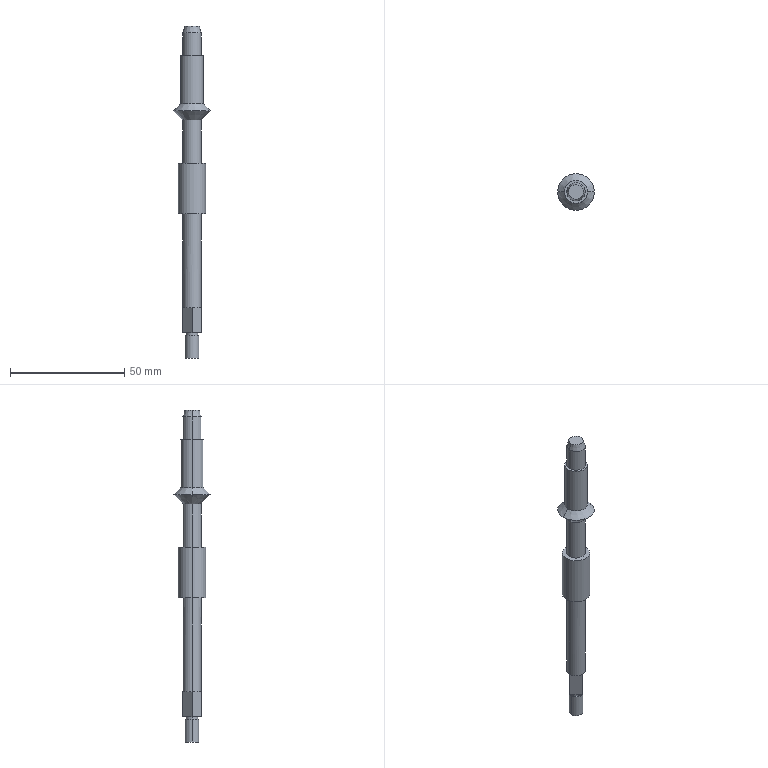Part | SolidWorks | features ICE 8, Chamfer 3, Extrusion 1 | 1 solid | 35 faces | box 16 x 16 x 145 mm | volume 9307 mm3 | plane 15 | cylinder 14 | cone 6 | commonest cylinder face diameters 8 x6 5 x2 6 x2 10 x2 12 x2
STEP:
#1=CARTESIAN_POINT('',(3.196,0.,145.));
#2=VERTEX_POINT('',#1);
#3=CARTESIAN_POINT('',(-3.196,0.,145.));
#4=VERTEX_POINT('',#3);
#5=CARTESIAN_POINT('',(0.,0.,145.));
#6=DIRECTION('',(0.,0.,1.));
#7=DIRECTION('',(1.,0.,0.));
#8=AXIS2_PLACEMENT_3D('',#5,#6,#7);
#9=CIRCLE('',#8,3.196);
#10=EDGE_CURVE('',#2,#4,#9,.T.);
#11=ORIENTED_EDGE('',*,*,#10,.F.);
#12=CARTESIAN_POINT('',(4.,0.,142.));
#13=VERTEX_POINT('',#12);
#14=CARTESIAN_POINT('',(3.196,0.,145.));
#15=DIRECTION('',(0.2588,0.,-0.9659));
#16=VECTOR('',#15,1000.);
#17=LINE('',#14,#16);
#18=EDGE_CURVE('',#2,#13,#17,.T.);
#19=ORIENTED_EDGE('',*,*,#18,.T.);
#20=CARTESIAN_POINT('',(-4.,0.,142.));
#21=VERTEX_POINT('',#20);
#22=CARTESIAN_POINT('',(0.,0.,142.));
#23=DIRECTION('',(0.,0.,-1.));
#24=DIRECTION('',(1.,0.,0.));
#25=AXIS2_PLACEMENT_3D('',#22,#23,#24);
#26=CIRCLE('',#25,4.);
#27=EDGE_CURVE('',#21,#13,#26,.T.);
#28=ORIENTED_EDGE('',*,*,#27,.F.);
#29=CARTESIAN_POINT('',(-3.196,0.,145.));
#30=DIRECTION('',(-0.2588,0.,-0.9659));
#31=VECTOR('',#30,1000.);
#32=LINE('',#29,#31);
#33=EDGE_CURVE('',#4,#21,#32,.T.);
#34=ORIENTED_EDGE('',*,*,#33,.F.);
#35=EDGE_LOOP('',(#11,#19,#28,#34));
#36=FACE_OUTER_BOUND('',#35,.T.);
#37=CARTESIAN_POINT('',(0.,0.,145.));
#38=DIRECTION('',(0.,0.,-1.));
#39=DIRECTION('',(-1.,0.,0.));
#40=AXIS2_PLACEMENT_3D('',#37,#38,#39);
#41=CONICAL_SURFACE('',#40,3.196,0.2618);
#42=ADVANCED_FACE('',(#36),#41,.T.);
#43=CARTESIAN_POINT('',(5.,0.,111.));
#44=VERTEX_POINT('',#43);
#45=CARTESIAN_POINT('',(-5.,0.,111.));
#46=VERTEX_POINT('',#45);
#47=CARTESIAN_POINT('',(0.,0.,111.));
#48=DIRECTION('',(0.,0.,1.));
#49=DIRECTION('',(-1.,0.,0.));
#50=AXIS2_PLACEMENT_3D('',#47,#48,#49);
#51=CIRCLE('',#50,5.);
#52=EDGE_CURVE('',#44,#46,#51,.T.);
#53=ORIENTED_EDGE('',*,*,#52,.F.);
#54=CARTESIAN_POINT('',(8.,0.,108.));
#55=VERTEX_POINT('',#54);
#56=CARTESIAN_POINT('',(4.,0.,112.));
#57=DIRECTION('',(0.7071,0.,-0.7071));
#58=VECTOR('',#57,1000.);
#59=LINE('',#56,#58);
#60=EDGE_CURVE('',#44,#55,#59,.T.);
#61=ORIENTED_EDGE('',*,*,#60,.T.);
#62=CARTESIAN_POINT('',(-8.,0.,108.));
#63=VERTEX_POINT('',#62);
#64=CARTESIAN_POINT('',(0.,0.,108.));
#65=DIRECTION('',(0.,0.,-1.));
#66=DIRECTION('',(-1.,0.,0.));
#67=AXIS2_PLACEMENT_3D('',#64,#65,#66);
#68=CIRCLE('',#67,8.);
#69=EDGE_CURVE('',#63,#55,#68,.T.);
#70=ORIENTED_EDGE('',*,*,#69,.F.);
#71=CARTESIAN_POINT('',(-4.,0.,112.));
#72=DIRECTION('',(-0.7071,0.,-0.7071));
#73=VECTOR('',#72,1000.);
#74=LINE('',#71,#73);
#75=EDGE_CURVE('',#46,#63,#74,.T.);
#76=ORIENTED_EDGE('',*,*,#75,.F.);
#77=EDGE_LOOP('',(#53,#61,#70,#76));
#78=FACE_OUTER_BOUND('',#77,.T.);
#79=CARTESIAN_POINT('',(0.,0.,112.));
#80=DIRECTION('',(0.,0.,-1.));
#81=DIRECTION('',(-1.,0.,0.));
#82=AXIS2_PLACEMENT_3D('',#79,#80,#81);
#83=CONICAL_SURFACE('',#82,4.,0.7854);
#84=ADVANCED_FACE('',(#78),#83,.T.);
#85=CARTESIAN_POINT('',(4.,0.,104.));
#86=VERTEX_POINT('',#85);
#87=CARTESIAN_POINT('',(-4.,0.,104.));
#88=VERTEX_POINT('',#87);
#89=CARTESIAN_POINT('',(0.,0.,104.));
#90=DIRECTION('',(0.,0.,1.));
#91=DIRECTION('',(1.,0.,0.));
#92=AXIS2_PLACEMENT_3D('',#89,#90,#91);
#93=CIRCLE('',#92,4.);
#94=EDGE_CURVE('',#86,#88,#93,.T.);
#95=ORIENTED_EDGE('',*,*,#94,.T.);
#96=CARTESIAN_POINT('',(-11.,0.,111.));
#97=DIRECTION('',(-0.7071,0.,0.7071));
#98=VECTOR('',#97,1000.);
#99=LINE('',#96,#98);
#100=EDGE_CURVE('',#88,#63,#99,.T.);
#101=ORIENTED_EDGE('',*,*,#100,.T.);
#102=ORIENTED_EDGE('',*,*,#69,.T.);
#103=CARTESIAN_POINT('',(11.,0.,111.));
#104=DIRECTION('',(0.7071,0.,0.7071));
#105=VECTOR('',#104,1000.);
#106=LINE('',#103,#105);
#107=EDGE_CURVE('',#86,#55,#106,.T.);
#108=ORIENTED_EDGE('',*,*,#107,.F.);
#109=EDGE_LOOP('',(#95,#101,#102,#108));
#110=FACE_OUTER_BOUND('',#109,.T.);
#111=CARTESIAN_POINT('',(0.,0.,111.));
#112=DIRECTION('',(0.,0.,1.));
#113=DIRECTION('',(1.,0.,0.));
#114=AXIS2_PLACEMENT_3D('',#111,#112,#113);
#115=CONICAL_SURFACE('',#114,11.,0.7854);
#116=ADVANCED_FACE('',(#110),#115,.T.);
#117=ORIENTED_EDGE('',*,*,#27,.T.);
#118=CARTESIAN_POINT('',(4.,0.,132.));
#119=VERTEX_POINT('',#118);
#120=CARTESIAN_POINT('',(4.,0.,145.));
#121=DIRECTION('',(0.,0.,-1.));
#122=VECTOR('',#121,1000.);
#123=LINE('',#120,#122);
#124=EDGE_CURVE('',#13,#119,#123,.T.);
#125=ORIENTED_EDGE('',*,*,#124,.T.);
#126=CARTESIAN_POINT('',(-4.,0.,132.));
#127=VERTEX_POINT('',#126);
#128=CARTESIAN_POINT('',(0.,0.,132.));
#129=DIRECTION('',(0.,0.,1.));
#130=DIRECTION('',(1.,0.,0.));
#131=AXIS2_PLACEMENT_3D('',#128,#129,#130);
#132=CIRCLE('',#131,4.);
#133=EDGE_CURVE('',#119,#127,#132,.T.);
#134=ORIENTED_EDGE('',*,*,#133,.T.);
#135=CARTESIAN_POINT('',(-4.,0.,145.));
#136=DIRECTION('',(0.,0.,-1.));
#137=VECTOR('',#136,1000.);
#138=LINE('',#135,#137);
#139=EDGE_CURVE('',#21,#127,#138,.T.);
#140=ORIENTED_EDGE('',*,*,#139,.F.);
#141=EDGE_LOOP('',(#117,#125,#134,#140));
#142=FACE_OUTER_BOUND('',#141,.T.);
#143=CARTESIAN_POINT('',(0.,0.,145.));
#144=DIRECTION('',(0.,0.,-1.));
#145=DIRECTION('',(-1.,0.,0.));
#146=AXIS2_PLACEMENT_3D('',#143,#144,#145);
#147=CYLINDRICAL_SURFACE('',#146,4.);
#148=ADVANCED_FACE('',(#142),#147,.T.);
#149=CARTESIAN_POINT('',(5.,0.,132.));
#150=VERTEX_POINT('',#149);
#151=CARTESIAN_POINT('',(-5.,0.,132.));
#152=VERTEX_POINT('',#151);
#153=CARTESIAN_POINT('',(0.,0.,132.));
#154=DIRECTION('',(0.,0.,1.));
#155=DIRECTION('',(1.,0.,0.));
#156=AXIS2_PLACEMENT_3D('',#153,#154,#155);
#157=CIRCLE('',#156,5.);
#158=EDGE_CURVE('',#150,#152,#157,.T.);
#159=ORIENTED_EDGE('',*,*,#158,.F.);
#160=CARTESIAN_POINT('',(5.,0.,132.));
#161=DIRECTION('',(0.,0.,-1.));
#162=VECTOR('',#161,1000.);
#163=LINE('',#160,#162);
#164=EDGE_CURVE('',#150,#44,#163,.T.);
#165=ORIENTED_EDGE('',*,*,#164,.T.);
#166=ORIENTED_EDGE('',*,*,#52,.T.);
#167=CARTESIAN_POINT('',(-5.,0.,132.));
#168=DIRECTION('',(0.,0.,-1.));
#169=VECTOR('',#168,1000.);
#170=LINE('',#167,#169);
#171=EDGE_CURVE('',#152,#46,#170,.T.);
#172=ORIENTED_EDGE('',*,*,#171,.F.);
#173=EDGE_LOOP('',(#159,#165,#166,#172));
#174=FACE_OUTER_BOUND('',#173,.T.);
#175=CARTESIAN_POINT('',(0.,0.,132.));
#176=DIRECTION('',(0.,0.,-1.));
#177=DIRECTION('',(-1.,0.,0.));
#178=AXIS2_PLACEMENT_3D('',#175,#176,#177);
#179=CYLINDRICAL_SURFACE('',#178,5.);
#180=ADVANCED_FACE('',(#174),#179,.T.);
#181=ORIENTED_EDGE('',*,*,#94,.F.);
#182=CARTESIAN_POINT('',(4.,0.,85.));
#183=VERTEX_POINT('',#182);
#184=CARTESIAN_POINT('',(4.,0.,104.));
#185=DIRECTION('',(0.,0.,-1.));
#186=VECTOR('',#185,1000.);
#187=LINE('',#184,#186);
#188=EDGE_CURVE('',#86,#183,#187,.T.);
#189=ORIENTED_EDGE('',*,*,#188,.T.);
#190=CARTESIAN_POINT('',(-4.,0.,85.));
#191=VERTEX_POINT('',#190);
#192=CARTESIAN_POINT('',(0.,0.,85.));
#193=DIRECTION('',(0.,0.,1.));
#194=DIRECTION('',(1.,0.,0.));
#195=AXIS2_PLACEMENT_3D('',#192,#193,#194);
#196=CIRCLE('',#195,4.);
#197=EDGE_CURVE('',#183,#191,#196,.T.);
#198=ORIENTED_EDGE('',*,*,#197,.T.);
#199=CARTESIAN_POINT('',(-4.,0.,104.));
#200=DIRECTION('',(0.,0.,-1.));
#201=VECTOR('',#200,1000.);
#202=LINE('',#199,#201);
#203=EDGE_CURVE('',#88,#191,#202,.T.);
#204=ORIENTED_EDGE('',*,*,#203,.F.);
#205=EDGE_LOOP('',(#181,#189,#198,#204));
#206=FACE_OUTER_BOUND('',#205,.T.);
#207=CARTESIAN_POINT('',(0.,0.,104.));
#208=DIRECTION('',(0.,0.,-1.));
#209=DIRECTION('',(-1.,0.,0.));
#210=AXIS2_PLACEMENT_3D('',#207,#208,#209);
#211=CYLINDRICAL_SURFACE('',#210,4.);
#212=ADVANCED_FACE('',(#206),#211,.T.);
#213=CARTESIAN_POINT('',(6.,0.,85.));
#214=VERTEX_POINT('',#213);
#215=CARTESIAN_POINT('',(-6.,0.,85.));
#216=VERTEX_POINT('',#215);
#217=CARTESIAN_POINT('',(0.,0.,85.));
#218=DIRECTION('',(0.,0.,1.));
#219=DIRECTION('',(1.,0.,0.));
#220=AXIS2_PLACEMENT_3D('',#217,#218,#219);
#221=CIRCLE('',#220,6.);
#222=EDGE_CURVE('',#214,#216,#221,.T.);
#223=ORIENTED_EDGE('',*,*,#222,.F.);
#224=CARTESIAN_POINT('',(6.,0.,63.));
#225=VERTEX_POINT('',#224);
#226=CARTESIAN_POINT('',(6.,0.,85.));
#227=DIRECTION('',(0.,0.,-1.));
#228=VECTOR('',#227,1000.);
#229=LINE('',#226,#228);
#230=EDGE_CURVE('',#214,#225,#229,.T.);
#231=ORIENTED_EDGE('',*,*,#230,.T.);
#232=CARTESIAN_POINT('',(-6.,0.,63.));
#233=VERTEX_POINT('',#232);
#234=CARTESIAN_POINT('',(0.,0.,63.));
#235=DIRECTION('',(0.,0.,1.));
#236=DIRECTION('',(1.,0.,0.));
#237=AXIS2_PLACEMENT_3D('',#234,#235,#236);
#238=CIRCLE('',#237,6.);
#239=EDGE_CURVE('',#225,#233,#238,.T.);
#240=ORIENTED_EDGE('',*,*,#239,.T.);
#241=CARTESIAN_POINT('',(-6.,0.,85.));
#242=DIRECTION('',(0.,0.,-1.));
#243=VECTOR('',#242,1000.);
#244=LINE('',#241,#243);
#245=EDGE_CURVE('',#216,#233,#244,.T.);
#246=ORIENTED_EDGE('',*,*,#245,.F.);
#247=EDGE_LOOP('',(#223,#231,#240,#246));
#248=FACE_OUTER_BOUND('',#247,.T.);
#249=CARTESIAN_POINT('',(0.,0.,85.));
#250=DIRECTION('',(0.,0.,-1.));
#251=DIRECTION('',(-1.,0.,0.));
#252=AXIS2_PLACEMENT_3D('',#249,#250,#251);
#253=CYLINDRICAL_SURFACE('',#252,6.);
#254=ADVANCED_FACE('',(#248),#253,.T.);
#255=CARTESIAN_POINT('',(2.5,0.,11.));
#256=VERTEX_POINT('',#255);
#257=CARTESIAN_POINT('',(-2.5,0.,11.));
#258=VERTEX_POINT('',#257);
#259=CARTESIAN_POINT('',(0.,0.,11.));
#260=DIRECTION('',(0.,0.,1.));
#261=DIRECTION('',(1.,0.,0.));
#262=AXIS2_PLACEMENT_3D('',#259,#260,#261);
#263=CIRCLE('',#262,2.5);
#264=EDGE_CURVE('',#256,#258,#263,.T.);
#265=ORIENTED_EDGE('',*,*,#264,.F.);
#266=CARTESIAN_POINT('',(2.5,0.,10.));
#267=VERTEX_POINT('',#266);
#268=CARTESIAN_POINT('',(2.5,0.,11.));
#269=DIRECTION('',(0.,0.,-1.));
#270=VECTOR('',#269,1000.);
#271=LINE('',#268,#270);
#272=EDGE_CURVE('',#256,#267,#271,.T.);
#273=ORIENTED_EDGE('',*,*,#272,.T.);
#274=CARTESIAN_POINT('',(-2.5,0.,10.));
#275=VERTEX_POINT('',#274);
#276=CARTESIAN_POINT('',(0.,0.,10.));
#277=DIRECTION('',(0.,0.,1.));
#278=DIRECTION('',(1.,0.,0.));
#279=AXIS2_PLACEMENT_3D('',#276,#277,#278);
#280=CIRCLE('',#279,2.5);
#281=EDGE_CURVE('',#267,#275,#280,.T.);
#282=ORIENTED_EDGE('',*,*,#281,.T.);
#283=CARTESIAN_POINT('',(-2.5,0.,11.));
#284=DIRECTION('',(0.,0.,-1.));
#285=VECTOR('',#284,1000.);
#286=LINE('',#283,#285);
#287=EDGE_CURVE('',#258,#275,#286,.T.);
#288=ORIENTED_EDGE('',*,*,#287,.F.);
#289=EDGE_LOOP('',(#265,#273,#282,#288));
#290=FACE_OUTER_BOUND('',#289,.T.);
#291=CARTESIAN_POINT('',(0.,0.,11.));
#292=DIRECTION('',(0.,0.,-1.));
#293=DIRECTION('',(-1.,0.,0.));
#294=AXIS2_PLACEMENT_3D('',#291,#292,#293);
#295=CYLINDRICAL_SURFACE('',#294,2.5);
#296=ADVANCED_FACE('',(#290),#295,.T.);
#297=CARTESIAN_POINT('',(3.,0.,10.));
#298=VERTEX_POINT('',#297);
#299=CARTESIAN_POINT('',(-3.,0.,10.));
#300=VERTEX_POINT('',#299);
#301=CARTESIAN_POINT('',(0.,0.,10.));
#302=DIRECTION('',(0.,0.,1.));
#303=DIRECTION('',(1.,0.,0.));
#304=AXIS2_PLACEMENT_3D('',#301,#302,#303);
#305=CIRCLE('',#304,3.);
#306=EDGE_CURVE('',#298,#300,#305,.T.);
#307=ORIENTED_EDGE('',*,*,#306,.F.);
#308=CARTESIAN_POINT('',(3.,0.,0.));
#309=VERTEX_POINT('',#308);
#310=CARTESIAN_POINT('',(3.,0.,10.));
#311=DIRECTION('',(0.,0.,-1.));
#312=VECTOR('',#311,1000.);
#313=LINE('',#310,#312);
#314=EDGE_CURVE('',#298,#309,#313,.T.);
#315=ORIENTED_EDGE('',*,*,#314,.T.);
#316=CARTESIAN_POINT('',(-3.,0.,0.));
#317=VERTEX_POINT('',#316);
#318=CARTESIAN_POINT('',(0.,0.,0.));
#319=DIRECTION('',(0.,0.,1.));
#320=DIRECTION('',(1.,0.,0.));
#321=AXIS2_PLACEMENT_3D('',#318,#319,#320);
#322=CIRCLE('',#321,3.);
#323=EDGE_CURVE('',#309,#317,#322,.T.);
#324=ORIENTED_EDGE('',*,*,#323,.T.);
#325=CARTESIAN_POINT('',(-3.,0.,10.));
#326=DIRECTION('',(0.,0.,-1.));
#327=VECTOR('',#326,1000.);
#328=LINE('',#325,#327);
#329=EDGE_CURVE('',#300,#317,#328,.T.);
#330=ORIENTED_EDGE('',*,*,#329,.F.);
#331=EDGE_LOOP('',(#307,#315,#324,#330));
#332=FACE_OUTER_BOUND('',#331,.T.);
#333=CARTESIAN_POINT('',(0.,0.,10.));
#334=DIRECTION('',(0.,0.,-1.));
#335=DIRECTION('',(-1.,0.,0.));
#336=AXIS2_PLACEMENT_3D('',#333,#334,#335);
#337=CYLINDRICAL_SURFACE('',#336,3.);
#338=ADVANCED_FACE('',(#332),#337,.T.);
#339=CARTESIAN_POINT('',(4.,0.,63.));
#340=VERTEX_POINT('',#339);
#341=CARTESIAN_POINT('',(-4.,0.,63.));
#342=VERTEX_POINT('',#341);
#343=CARTESIAN_POINT('',(0.,0.,63.));
#344=DIRECTION('',(0.,0.,1.));
#345=DIRECTION('',(1.,0.,0.));
#346=AXIS2_PLACEMENT_3D('',#343,#344,#345);
#347=CIRCLE('',#346,4.);
#348=EDGE_CURVE('',#340,#342,#347,.T.);
#349=ORIENTED_EDGE('',*,*,#348,.F.);
#350=CARTESIAN_POINT('',(4.,0.,22.));
#351=VERTEX_POINT('',#350);
#352=CARTESIAN_POINT('',(4.,0.,63.));
#353=DIRECTION('',(0.,0.,-1.));
#354=VECTOR('',#353,1000.);
#355=LINE('',#352,#354);
#356=EDGE_CURVE('',#340,#351,#355,.T.);
#357=ORIENTED_EDGE('',*,*,#356,.T.);
#358=CARTESIAN_POINT('',(0.,4.,22.));
#359=VERTEX_POINT('',#358);
#360=CARTESIAN_POINT('',(0.,0.,22.));
#361=DIRECTION('',(0.,0.,-1.));
#362=DIRECTION('',(-1.,0.,0.));
#363=AXIS2_PLACEMENT_3D('',#360,#361,#362);
#364=CIRCLE('',#363,4.);
#365=EDGE_CURVE('',#359,#351,#364,.T.);
#366=ORIENTED_EDGE('',*,*,#365,.F.);
#367=CARTESIAN_POINT('',(-4.,0.,22.));
#368=VERTEX_POINT('',#367);
#369=CARTESIAN_POINT('',(0.,0.,22.));
#370=DIRECTION('',(0.,0.,-1.));
#371=DIRECTION('',(-1.,0.,0.));
#372=AXIS2_PLACEMENT_3D('',#369,#370,#371);
#373=CIRCLE('',#372,4.);
#374=EDGE_CURVE('',#368,#359,#373,.T.);
#375=ORIENTED_EDGE('',*,*,#374,.F.);
#376=CARTESIAN_POINT('',(-4.,0.,63.));
#377=DIRECTION('',(0.,0.,-1.));
#378=VECTOR('',#377,1000.);
#379=LINE('',#376,#378);
#380=EDGE_CURVE('',#342,#368,#379,.T.);
#381=ORIENTED_EDGE('',*,*,#380,.F.);
#382=EDGE_LOOP('',(#349,#357,#366,#375,#381));
#383=FACE_OUTER_BOUND('',#382,.T.);
#384=CARTESIAN_POINT('',(0.,0.,63.));
#385=DIRECTION('',(0.,0.,-1.));
#386=DIRECTION('',(-1.,0.,0.));
#387=AXIS2_PLACEMENT_3D('',#384,#385,#386);
#388=CYLINDRICAL_SURFACE('',#387,4.);
#389=ADVANCED_FACE('',(#383),#388,.T.);
#390=ORIENTED_EDGE('',*,*,#356,.F.);
#391=CARTESIAN_POINT('',(0.,0.,63.));
#392=DIRECTION('',(0.,0.,1.));
#393=DIRECTION('',(1.,0.,0.));
#394=AXIS2_PLACEMENT_3D('',#391,#392,#393);
#395=CIRCLE('',#394,4.);
#396=EDGE_CURVE('',#342,#340,#395,.T.);
#397=ORIENTED_EDGE('',*,*,#396,.F.);
#398=ORIENTED_EDGE('',*,*,#380,.T.);
#399=CARTESIAN_POINT('',(0.,-4.,22.));
#400=VERTEX_POINT('',#399);
#401=CARTESIAN_POINT('',(0.,0.,22.));
#402=DIRECTION('',(0.,0.,-1.));
#403=DIRECTION('',(-1.,0.,0.));
#404=AXIS2_PLACEMENT_3D('',#401,#402,#403);
#405=CIRCLE('',#404,4.);
#406=EDGE_CURVE('',#400,#368,#405,.T.);
#407=ORIENTED_EDGE('',*,*,#406,.F.);
#408=CARTESIAN_POINT('',(0.,0.,22.));
#409=DIRECTION('',(0.,0.,-1.));
#410=DIRECTION('',(-1.,0.,0.));
#411=AXIS2_PLACEMENT_3D('',#408,#409,#410);
#412=CIRCLE('',#411,4.);
#413=EDGE_CURVE('',#351,#400,#412,.T.);
#414=ORIENTED_EDGE('',*,*,#413,.F.);
#415=EDGE_LOOP('',(#390,#397,#398,#407,#414));
#416=FACE_OUTER_BOUND('',#415,.T.);
#417=CARTESIAN_POINT('',(0.,0.,63.));
#418=DIRECTION('',(0.,0.,-1.));
#419=DIRECTION('',(-1.,0.,0.));
#420=AXIS2_PLACEMENT_3D('',#417,#418,#419);
#421=CYLINDRICAL_SURFACE('',#420,4.);
#422=ADVANCED_FACE('',(#416),#421,.T.);
#423=CARTESIAN_POINT('',(0.,0.,11.));
#424=DIRECTION('',(0.,0.,1.));
#425=DIRECTION('',(1.,0.,0.));
#426=AXIS2_PLACEMENT_3D('',#423,#424,#425);
#427=CIRCLE('',#426,2.5);
#428=EDGE_CURVE('',#258,#256,#427,.T.);
#429=ORIENTED_EDGE('',*,*,#428,.T.);
#430=ORIENTED_EDGE('',*,*,#264,.T.);
#431=EDGE_LOOP('',(#429,#430));
#432=FACE_BOUND('',#431,.T.);
#433=CARTESIAN_POINT('',(0.,-4.,11.));
#434=VERTEX_POINT('',#433);
#435=CARTESIAN_POINT('',(-4.,0.,11.));
#436=VERTEX_POINT('',#435);
#437=CARTESIAN_POINT('',(-2.,-2.,11.));
#438=DIRECTION('',(-0.7071,0.7071,0.));
#439=VECTOR('',#438,1000.);
#440=LINE('',#437,#439);
#441=EDGE_CURVE('',#434,#436,#440,.T.);
#442=ORIENTED_EDGE('',*,*,#441,.T.);
#443=CARTESIAN_POINT('',(0.,4.,11.));
#444=VERTEX_POINT('',#443);
#445=CARTESIAN_POINT('',(-2.,2.,11.));
#446=DIRECTION('',(-0.7071,-0.7071,0.));
#447=VECTOR('',#446,1000.);
#448=LINE('',#445,#447);
#449=EDGE_CURVE('',#444,#436,#448,.T.);
#450=ORIENTED_EDGE('',*,*,#449,.F.);
#451=CARTESIAN_POINT('',(4.,0.,11.));
#452=VERTEX_POINT('',#451);
#453=CARTESIAN_POINT('',(2.,2.,11.));
#454=DIRECTION('',(-0.7071,0.7071,0.));
#455=VECTOR('',#454,1000.);
#456=LINE('',#453,#455);
#457=EDGE_CURVE('',#452,#444,#456,.T.);
#458=ORIENTED_EDGE('',*,*,#457,.F.);
#459=CARTESIAN_POINT('',(2.,-2.,11.));
#460=DIRECTION('',(-0.7071,-0.7071,0.));
#461=VECTOR('',#460,1000.);
#462=LINE('',#459,#461);
#463=EDGE_CURVE('',#452,#434,#462,.T.);
#464=ORIENTED_EDGE('',*,*,#463,.T.);
#465=EDGE_LOOP('',(#442,#450,#458,#464));
#466=FACE_OUTER_BOUND('',#465,.T.);
#467=CARTESIAN_POINT('',(0.,0.,11.));
#468=DIRECTION('',(0.,0.,1.));
#469=DIRECTION('',(1.,0.,0.));
#470=AXIS2_PLACEMENT_3D('',#467,#468,#469);
#471=PLANE('',#470);
#472=ADVANCED_FACE('',(#432,#466),#471,.F.);
#473=ORIENTED_EDGE('',*,*,#314,.F.);
#474=CARTESIAN_POINT('',(0.,0.,10.));
#475=DIRECTION('',(0.,0.,1.));
#476=DIRECTION('',(1.,0.,0.));
#477=AXIS2_PLACEMENT_3D('',#474,#475,#476);
#478=CIRCLE('',#477,3.);
#479=EDGE_CURVE('',#300,#298,#478,.T.);
#480=ORIENTED_EDGE('',*,*,#479,.F.);
#481=ORIENTED_EDGE('',*,*,#329,.T.);
#482=CARTESIAN_POINT('',(0.,0.,0.));
#483=DIRECTION('',(0.,0.,1.));
#484=DIRECTION('',(1.,0.,0.));
#485=AXIS2_PLACEMENT_3D('',#482,#483,#484);
#486=CIRCLE('',#485,3.);
#487=EDGE_CURVE('',#317,#309,#486,.T.);
#488=ORIENTED_EDGE('',*,*,#487,.T.);
#489=EDGE_LOOP('',(#473,#480,#481,#488));
#490=FACE_OUTER_BOUND('',#489,.T.);
#491=CARTESIAN_POINT('',(0.,0.,10.));
#492=DIRECTION('',(0.,0.,-1.));
#493=DIRECTION('',(-1.,0.,0.));
#494=AXIS2_PLACEMENT_3D('',#491,#492,#493);
#495=CYLINDRICAL_SURFACE('',#494,3.);
#496=ADVANCED_FACE('',(#490),#495,.T.);
#497=CARTESIAN_POINT('',(0.,0.,10.));
#498=DIRECTION('',(0.,0.,1.));
#499=DIRECTION('',(1.,0.,0.));
#500=AXIS2_PLACEMENT_3D('',#497,#498,#499);
#501=CIRCLE('',#500,2.5);
#502=EDGE_CURVE('',#275,#267,#501,.T.);
#503=ORIENTED_EDGE('',*,*,#502,.F.);
#504=ORIENTED_EDGE('',*,*,#281,.F.);
#505=EDGE_LOOP('',(#503,#504));
#506=FACE_BOUND('',#505,.T.);
#507=ORIENTED_EDGE('',*,*,#479,.T.);
#508=ORIENTED_EDGE('',*,*,#306,.T.);
#509=EDGE_LOOP('',(#507,#508));
#510=FACE_OUTER_BOUND('',#509,.T.);
#511=CARTESIAN_POINT('',(0.,0.,10.));
#512=DIRECTION('',(0.,0.,1.));
#513=DIRECTION('',(1.,0.,0.));
#514=AXIS2_PLACEMENT_3D('',#511,#512,#513);
#515=PLANE('',#514);
#516=ADVANCED_FACE('',(#506,#510),#515,.T.);
#517=ORIENTED_EDGE('',*,*,#487,.F.);
#518=ORIENTED_EDGE('',*,*,#323,.F.);
#519=EDGE_LOOP('',(#517,#518));
#520=FACE_OUTER_BOUND('',#519,.T.);
#521=CARTESIAN_POINT('',(0.,0.,0.));
#522=DIRECTION('',(0.,0.,1.));
#523=DIRECTION('',(1.,0.,0.));
#524=AXIS2_PLACEMENT_3D('',#521,#522,#523);
#525=PLANE('',#524);
#526=ADVANCED_FACE('',(#520),#525,.F.);
#527=ORIENTED_EDGE('',*,*,#272,.F.);
#528=ORIENTED_EDGE('',*,*,#428,.F.);
#529=ORIENTED_EDGE('',*,*,#287,.T.);
#530=ORIENTED_EDGE('',*,*,#502,.T.);
#531=EDGE_LOOP('',(#527,#528,#529,#530));
#532=FACE_OUTER_BOUND('',#531,.T.);
#533=CARTESIAN_POINT('',(0.,0.,11.));
#534=DIRECTION('',(0.,0.,-1.));
#535=DIRECTION('',(-1.,0.,0.));
#536=AXIS2_PLACEMENT_3D('',#533,#534,#535);
#537=CYLINDRICAL_SURFACE('',#536,2.5);
#538=ADVANCED_FACE('',(#532),#537,.T.);
#539=ORIENTED_EDGE('',*,*,#230,.F.);
#540=CARTESIAN_POINT('',(0.,0.,85.));
#541=DIRECTION('',(0.,0.,1.));
#542=DIRECTION('',(1.,0.,0.));
#543=AXIS2_PLACEMENT_3D('',#540,#541,#542);
#544=CIRCLE('',#543,6.);
#545=EDGE_CURVE('',#216,#214,#544,.T.);
#546=ORIENTED_EDGE('',*,*,#545,.F.);
#547=ORIENTED_EDGE('',*,*,#245,.T.);
#548=CARTESIAN_POINT('',(0.,0.,63.));
#549=DIRECTION('',(0.,0.,1.));
#550=DIRECTION('',(1.,0.,0.));
#551=AXIS2_PLACEMENT_3D('',#548,#549,#550);
#552=CIRCLE('',#551,6.);
#553=EDGE_CURVE('',#233,#225,#552,.T.);
#554=ORIENTED_EDGE('',*,*,#553,.T.);
#555=EDGE_LOOP('',(#539,#546,#547,#554));
#556=FACE_OUTER_BOUND('',#555,.T.);
#557=CARTESIAN_POINT('',(0.,0.,85.));
#558=DIRECTION('',(0.,0.,-1.));
#559=DIRECTION('',(-1.,0.,0.));
#560=AXIS2_PLACEMENT_3D('',#557,#558,#559);
#561=CYLINDRICAL_SURFACE('',#560,6.);
#562=ADVANCED_FACE('',(#556),#561,.T.);
#563=CARTESIAN_POINT('',(0.,0.,85.));
#564=DIRECTION('',(0.,0.,1.));
#565=DIRECTION('',(1.,0.,0.));
#566=AXIS2_PLACEMENT_3D('',#563,#564,#565);
#567=CIRCLE('',#566,4.);
#568=EDGE_CURVE('',#191,#183,#567,.T.);
#569=ORIENTED_EDGE('',*,*,#568,.F.);
#570=ORIENTED_EDGE('',*,*,#197,.F.);
#571=EDGE_LOOP('',(#569,#570));
#572=FACE_BOUND('',#571,.T.);
#573=ORIENTED_EDGE('',*,*,#545,.T.);
#574=ORIENTED_EDGE('',*,*,#222,.T.);
#575=EDGE_LOOP('',(#573,#574));
#576=FACE_OUTER_BOUND('',#575,.T.);
#577=CARTESIAN_POINT('',(0.,0.,85.));
#578=DIRECTION('',(0.,0.,1.));
#579=DIRECTION('',(1.,0.,0.));
#580=AXIS2_PLACEMENT_3D('',#577,#578,#579);
#581=PLANE('',#580);
#582=ADVANCED_FACE('',(#572,#576),#581,.T.);
#583=ORIENTED_EDGE('',*,*,#396,.T.);
#584=ORIENTED_EDGE('',*,*,#348,.T.);
#585=EDGE_LOOP('',(#583,#584));
#586=FACE_BOUND('',#585,.T.);
#587=ORIENTED_EDGE('',*,*,#553,.F.);
#588=ORIENTED_EDGE('',*,*,#239,.F.);
#589=EDGE_LOOP('',(#587,#588));
#590=FACE_OUTER_BOUND('',#589,.T.);
#591=CARTESIAN_POINT('',(0.,0.,63.));
#592=DIRECTION('',(0.,0.,1.));
#593=DIRECTION('',(1.,0.,0.));
#594=AXIS2_PLACEMENT_3D('',#591,#592,#593);
#595=PLANE('',#594);
#596=ADVANCED_FACE('',(#586,#590),#595,.F.);
#597=ORIENTED_EDGE('',*,*,#188,.F.);
#598=CARTESIAN_POINT('',(0.,0.,104.));
#599=DIRECTION('',(0.,0.,1.));
#600=DIRECTION('',(1.,0.,0.));
#601=AXIS2_PLACEMENT_3D('',#598,#599,#600);
#602=CIRCLE('',#601,4.);
#603=EDGE_CURVE('',#88,#86,#602,.T.);
#604=ORIENTED_EDGE('',*,*,#603,.F.);
#605=ORIENTED_EDGE('',*,*,#203,.T.);
#606=ORIENTED_EDGE('',*,*,#568,.T.);
#607=EDGE_LOOP('',(#597,#604,#605,#606));
#608=FACE_OUTER_BOUND('',#607,.T.);
#609=CARTESIAN_POINT('',(0.,0.,104.));
#610=DIRECTION('',(0.,0.,-1.));
#611=DIRECTION('',(-1.,0.,0.));
#612=AXIS2_PLACEMENT_3D('',#609,#610,#611);
#613=CYLINDRICAL_SURFACE('',#612,4.);
#614=ADVANCED_FACE('',(#608),#613,.T.);
#615=ORIENTED_EDGE('',*,*,#164,.F.);
#616=CARTESIAN_POINT('',(0.,0.,132.));
#617=DIRECTION('',(0.,0.,1.));
#618=DIRECTION('',(1.,0.,0.));
#619=AXIS2_PLACEMENT_3D('',#616,#617,#618);
#620=CIRCLE('',#619,5.);
#621=EDGE_CURVE('',#152,#150,#620,.T.);
#622=ORIENTED_EDGE('',*,*,#621,.F.);
#623=ORIENTED_EDGE('',*,*,#171,.T.);
#624=CARTESIAN_POINT('',(0.,0.,111.));
#625=DIRECTION('',(0.,0.,1.));
#626=DIRECTION('',(-1.,0.,0.));
#627=AXIS2_PLACEMENT_3D('',#624,#625,#626);
#628=CIRCLE('',#627,5.);
#629=EDGE_CURVE('',#46,#44,#628,.T.);
#630=ORIENTED_EDGE('',*,*,#629,.T.);
#631=EDGE_LOOP('',(#615,#622,#623,#630));
#632=FACE_OUTER_BOUND('',#631,.T.);
#633=CARTESIAN_POINT('',(0.,0.,132.));
#634=DIRECTION('',(0.,0.,-1.));
#635=DIRECTION('',(-1.,0.,0.));
#636=AXIS2_PLACEMENT_3D('',#633,#634,#635);
#637=CYLINDRICAL_SURFACE('',#636,5.);
#638=ADVANCED_FACE('',(#632),#637,.T.);
#639=CARTESIAN_POINT('',(0.,0.,132.));
#640=DIRECTION('',(0.,0.,1.));
#641=DIRECTION('',(1.,0.,0.));
#642=AXIS2_PLACEMENT_3D('',#639,#640,#641);
#643=CIRCLE('',#642,4.);
#644=EDGE_CURVE('',#127,#119,#643,.T.);
#645=ORIENTED_EDGE('',*,*,#644,.F.);
#646=ORIENTED_EDGE('',*,*,#133,.F.);
#647=EDGE_LOOP('',(#645,#646));
#648=FACE_BOUND('',#647,.T.);
#649=ORIENTED_EDGE('',*,*,#621,.T.);
#650=ORIENTED_EDGE('',*,*,#158,.T.);
#651=EDGE_LOOP('',(#649,#650));
#652=FACE_OUTER_BOUND('',#651,.T.);
#653=CARTESIAN_POINT('',(0.,0.,132.));
#654=DIRECTION('',(0.,0.,1.));
#655=DIRECTION('',(1.,0.,0.));
#656=AXIS2_PLACEMENT_3D('',#653,#654,#655);
#657=PLANE('',#656);
#658=ADVANCED_FACE('',(#648,#652),#657,.T.);
#659=CARTESIAN_POINT('',(0.,0.,145.));
#660=DIRECTION('',(0.,0.,1.));
#661=DIRECTION('',(1.,0.,0.));
#662=AXIS2_PLACEMENT_3D('',#659,#660,#661);
#663=CIRCLE('',#662,3.196);
#664=EDGE_CURVE('',#4,#2,#663,.T.);
#665=ORIENTED_EDGE('',*,*,#664,.T.);
#666=ORIENTED_EDGE('',*,*,#10,.T.);
#667=EDGE_LOOP('',(#665,#666));
#668=FACE_OUTER_BOUND('',#667,.T.);
#669=CARTESIAN_POINT('',(0.,0.,145.));
#670=DIRECTION('',(0.,0.,1.));
#671=DIRECTION('',(1.,0.,0.));
#672=AXIS2_PLACEMENT_3D('',#669,#670,#671);
#673=PLANE('',#672);
#674=ADVANCED_FACE('',(#668),#673,.T.);
#675=ORIENTED_EDGE('',*,*,#124,.F.);
#676=CARTESIAN_POINT('',(0.,0.,142.));
#677=DIRECTION('',(0.,0.,-1.));
#678=DIRECTION('',(1.,0.,0.));
#679=AXIS2_PLACEMENT_3D('',#676,#677,#678);
#680=CIRCLE('',#679,4.);
#681=EDGE_CURVE('',#13,#21,#680,.T.);
#682=ORIENTED_EDGE('',*,*,#681,.T.);
#683=ORIENTED_EDGE('',*,*,#139,.T.);
#684=ORIENTED_EDGE('',*,*,#644,.T.);
#685=EDGE_LOOP('',(#675,#682,#683,#684));
#686=FACE_OUTER_BOUND('',#685,.T.);
#687=CARTESIAN_POINT('',(0.,0.,145.));
#688=DIRECTION('',(0.,0.,-1.));
#689=DIRECTION('',(-1.,0.,0.));
#690=AXIS2_PLACEMENT_3D('',#687,#688,#689);
#691=CYLINDRICAL_SURFACE('',#690,4.);
#692=ADVANCED_FACE('',(#686),#691,.T.);
#693=ORIENTED_EDGE('',*,*,#100,.F.);
#694=ORIENTED_EDGE('',*,*,#603,.T.);
#695=ORIENTED_EDGE('',*,*,#107,.T.);
#696=CARTESIAN_POINT('',(0.,0.,108.));
#697=DIRECTION('',(0.,0.,-1.));
#698=DIRECTION('',(-1.,0.,0.));
#699=AXIS2_PLACEMENT_3D('',#696,#697,#698);
#700=CIRCLE('',#699,8.);
#701=EDGE_CURVE('',#55,#63,#700,.T.);
#702=ORIENTED_EDGE('',*,*,#701,.T.);
#703=EDGE_LOOP('',(#693,#694,#695,#702));
#704=FACE_OUTER_BOUND('',#703,.T.);
#705=CARTESIAN_POINT('',(0.,0.,111.));
#706=DIRECTION('',(0.,0.,1.));
#707=DIRECTION('',(1.,0.,0.));
#708=AXIS2_PLACEMENT_3D('',#705,#706,#707);
#709=CONICAL_SURFACE('',#708,11.,0.7854);
#710=ADVANCED_FACE('',(#704),#709,.T.);
#711=ORIENTED_EDGE('',*,*,#60,.F.);
#712=ORIENTED_EDGE('',*,*,#629,.F.);
#713=ORIENTED_EDGE('',*,*,#75,.T.);
#714=ORIENTED_EDGE('',*,*,#701,.F.);
#715=EDGE_LOOP('',(#711,#712,#713,#714));
#716=FACE_OUTER_BOUND('',#715,.T.);
#717=CARTESIAN_POINT('',(0.,0.,112.));
#718=DIRECTION('',(0.,0.,-1.));
#719=DIRECTION('',(-1.,0.,0.));
#720=AXIS2_PLACEMENT_3D('',#717,#718,#719);
#721=CONICAL_SURFACE('',#720,4.,0.7854);
#722=ADVANCED_FACE('',(#716),#721,.T.);
#723=ORIENTED_EDGE('',*,*,#18,.F.);
#724=ORIENTED_EDGE('',*,*,#664,.F.);
#725=ORIENTED_EDGE('',*,*,#33,.T.);
#726=ORIENTED_EDGE('',*,*,#681,.F.);
#727=EDGE_LOOP('',(#723,#724,#725,#726));
#728=FACE_OUTER_BOUND('',#727,.T.);
#729=CARTESIAN_POINT('',(0.,0.,145.));
#730=DIRECTION('',(0.,0.,-1.));
#731=DIRECTION('',(-1.,0.,0.));
#732=AXIS2_PLACEMENT_3D('',#729,#730,#731);
#733=CONICAL_SURFACE('',#732,3.196,0.2618);
#734=ADVANCED_FACE('',(#728),#733,.T.);
#735=ORIENTED_EDGE('',*,*,#449,.T.);
#736=CARTESIAN_POINT('',(-4.,0.,22.));
#737=DIRECTION('',(0.,0.,-1.));
#738=VECTOR('',#737,1000.);
#739=LINE('',#736,#738);
#740=EDGE_CURVE('',#368,#436,#739,.T.);
#741=ORIENTED_EDGE('',*,*,#740,.F.);
#742=CARTESIAN_POINT('',(-2.,2.,22.));
#743=DIRECTION('',(-0.7071,-0.7071,0.));
#744=VECTOR('',#743,1000.);
#745=LINE('',#742,#744);
#746=EDGE_CURVE('',#359,#368,#745,.T.);
#747=ORIENTED_EDGE('',*,*,#746,.F.);
#748=CARTESIAN_POINT('',(0.,4.,22.));
#749=DIRECTION('',(0.,0.,-1.));
#750=VECTOR('',#749,1000.);
#751=LINE('',#748,#750);
#752=EDGE_CURVE('',#359,#444,#751,.T.);
#753=ORIENTED_EDGE('',*,*,#752,.T.);
#754=EDGE_LOOP('',(#735,#741,#747,#753));
#755=FACE_OUTER_BOUND('',#754,.T.);
#756=CARTESIAN_POINT('',(-2.,2.,22.));
#757=DIRECTION('',(0.7071,-0.7071,0.));
#758=DIRECTION('',(0.7071,0.7071,0.));
#759=AXIS2_PLACEMENT_3D('',#756,#757,#758);
#760=PLANE('',#759);
#761=ADVANCED_FACE('',(#755),#760,.F.);
#762=ORIENTED_EDGE('',*,*,#374,.T.);
#763=ORIENTED_EDGE('',*,*,#746,.T.);
#764=EDGE_LOOP('',(#762,#763));
#765=FACE_OUTER_BOUND('',#764,.T.);
#766=CARTESIAN_POINT('',(0.,0.,22.));
#767=DIRECTION('',(0.,0.,-1.));
#768=DIRECTION('',(-1.,0.,0.));
#769=AXIS2_PLACEMENT_3D('',#766,#767,#768);
#770=PLANE('',#769);
#771=ADVANCED_FACE('',(#765),#770,.T.);
#772=ORIENTED_EDGE('',*,*,#463,.F.);
#773=CARTESIAN_POINT('',(4.,0.,22.));
#774=DIRECTION('',(0.,0.,-1.));
#775=VECTOR('',#774,1000.);
#776=LINE('',#773,#775);
#777=EDGE_CURVE('',#351,#452,#776,.T.);
#778=ORIENTED_EDGE('',*,*,#777,.F.);
#779=CARTESIAN_POINT('',(2.,-2.,22.));
#780=DIRECTION('',(-0.7071,-0.7071,0.));
#781=VECTOR('',#780,1000.);
#782=LINE('',#779,#781);
#783=EDGE_CURVE('',#351,#400,#782,.T.);
#784=ORIENTED_EDGE('',*,*,#783,.T.);
#785=CARTESIAN_POINT('',(0.,-4.,22.));
#786=DIRECTION('',(0.,0.,-1.));
#787=VECTOR('',#786,1000.);
#788=LINE('',#785,#787);
#789=EDGE_CURVE('',#400,#434,#788,.T.);
#790=ORIENTED_EDGE('',*,*,#789,.T.);
#791=EDGE_LOOP('',(#772,#778,#784,#790));
#792=FACE_OUTER_BOUND('',#791,.T.);
#793=CARTESIAN_POINT('',(2.,-2.,22.));
#794=DIRECTION('',(0.7071,-0.7071,0.));
#795=DIRECTION('',(0.7071,0.7071,0.));
#796=AXIS2_PLACEMENT_3D('',#793,#794,#795);
#797=PLANE('',#796);
#798=ADVANCED_FACE('',(#792),#797,.T.);
#799=ORIENTED_EDGE('',*,*,#783,.F.);
#800=ORIENTED_EDGE('',*,*,#413,.T.);
#801=EDGE_LOOP('',(#799,#800));
#802=FACE_OUTER_BOUND('',#801,.T.);
#803=CARTESIAN_POINT('',(0.,0.,22.));
#804=DIRECTION('',(0.,0.,-1.));
#805=DIRECTION('',(-1.,0.,0.));
#806=AXIS2_PLACEMENT_3D('',#803,#804,#805);
#807=PLANE('',#806);
#808=ADVANCED_FACE('',(#802),#807,.T.);
#809=ORIENTED_EDGE('',*,*,#457,.T.);
#810=ORIENTED_EDGE('',*,*,#752,.F.);
#811=CARTESIAN_POINT('',(2.,2.,22.));
#812=DIRECTION('',(-0.7071,0.7071,0.));
#813=VECTOR('',#812,1000.);
#814=LINE('',#811,#813);
#815=EDGE_CURVE('',#351,#359,#814,.T.);
#816=ORIENTED_EDGE('',*,*,#815,.F.);
#817=ORIENTED_EDGE('',*,*,#777,.T.);
#818=EDGE_LOOP('',(#809,#810,#816,#817));
#819=FACE_OUTER_BOUND('',#818,.T.);
#820=CARTESIAN_POINT('',(2.,2.,22.));
#821=DIRECTION('',(-0.7071,-0.7071,0.));
#822=DIRECTION('',(0.7071,-0.7071,0.));
#823=AXIS2_PLACEMENT_3D('',#820,#821,#822);
#824=PLANE('',#823);
#825=ADVANCED_FACE('',(#819),#824,.F.);
#826=ORIENTED_EDGE('',*,*,#365,.T.);
#827=ORIENTED_EDGE('',*,*,#815,.T.);
#828=EDGE_LOOP('',(#826,#827));
#829=FACE_OUTER_BOUND('',#828,.T.);
#830=CARTESIAN_POINT('',(0.,0.,22.));
#831=DIRECTION('',(0.,0.,-1.));
#832=DIRECTION('',(-1.,0.,0.));
#833=AXIS2_PLACEMENT_3D('',#830,#831,#832);
#834=PLANE('',#833);
#835=ADVANCED_FACE('',(#829),#834,.T.);
#836=ORIENTED_EDGE('',*,*,#441,.F.);
#837=ORIENTED_EDGE('',*,*,#789,.F.);
#838=CARTESIAN_POINT('',(-2.,-2.,22.));
#839=DIRECTION('',(-0.7071,0.7071,0.));
#840=VECTOR('',#839,1000.);
#841=LINE('',#838,#840);
#842=EDGE_CURVE('',#400,#368,#841,.T.);
#843=ORIENTED_EDGE('',*,*,#842,.T.);
#844=ORIENTED_EDGE('',*,*,#740,.T.);
#845=EDGE_LOOP('',(#836,#837,#843,#844));
#846=FACE_OUTER_BOUND('',#845,.T.);
#847=CARTESIAN_POINT('',(-2.,-2.,22.));
#848=DIRECTION('',(-0.7071,-0.7071,0.));
#849=DIRECTION('',(0.7071,-0.7071,0.));
#850=AXIS2_PLACEMENT_3D('',#847,#848,#849);
#851=PLANE('',#850);
#852=ADVANCED_FACE('',(#846),#851,.T.);
#853=ORIENTED_EDGE('',*,*,#842,.F.);
#854=ORIENTED_EDGE('',*,*,#406,.T.);
#855=EDGE_LOOP('',(#853,#854));
#856=FACE_OUTER_BOUND('',#855,.T.);
#857=CARTESIAN_POINT('',(0.,0.,22.));
#858=DIRECTION('',(0.,0.,-1.));
#859=DIRECTION('',(-1.,0.,0.));
#860=AXIS2_PLACEMENT_3D('',#857,#858,#859);
#861=PLANE('',#860);
#862=ADVANCED_FACE('',(#856),#861,.T.);
#863=CLOSED_SHELL('',(#42,#84,#116,#148,#180,#212,#254,#296,#338,#389,#422,#472,#496,#516,#526,#538,#562,#582,#596,#614,#638,#658,#674,#692,#710,#722,#734,#761,#771,#798,#808,#825,#835,#852,#862));
#864=MANIFOLD_SOLID_BREP('',#863);
#865=CARTESIAN_POINT('',(0.,0.,0.));
#866=DIRECTION('',(0.,0.,1.));
#867=DIRECTION('',(1.,0.,0.));
#868=AXIS2_PLACEMENT_3D('',#865,#866,#867);
#869=(LENGTH_UNIT()NAMED_UNIT(*)SI_UNIT(.MILLI.,.METRE.));
#870=UNCERTAINTY_MEASURE_WITH_UNIT(LENGTH_MEASURE(0.00001),#869,'','');
#871=(NAMED_UNIT(*)PLANE_ANGLE_UNIT()SI_UNIT($,.RADIAN.));
#872=(NAMED_UNIT(*)SI_UNIT($,.STERADIAN.)SOLID_ANGLE_UNIT());
#873=(GEOMETRIC_REPRESENTATION_CONTEXT(3)GLOBAL_UNCERTAINTY_ASSIGNED_CONTEXT((#870))GLOBAL_UNIT_ASSIGNED_CONTEXT((#869,#871,#872))REPRESENTATION_CONTEXT('',''));
#874=ADVANCED_BREP_SHAPE_REPRESENTATION('',(#864,#868),#873);